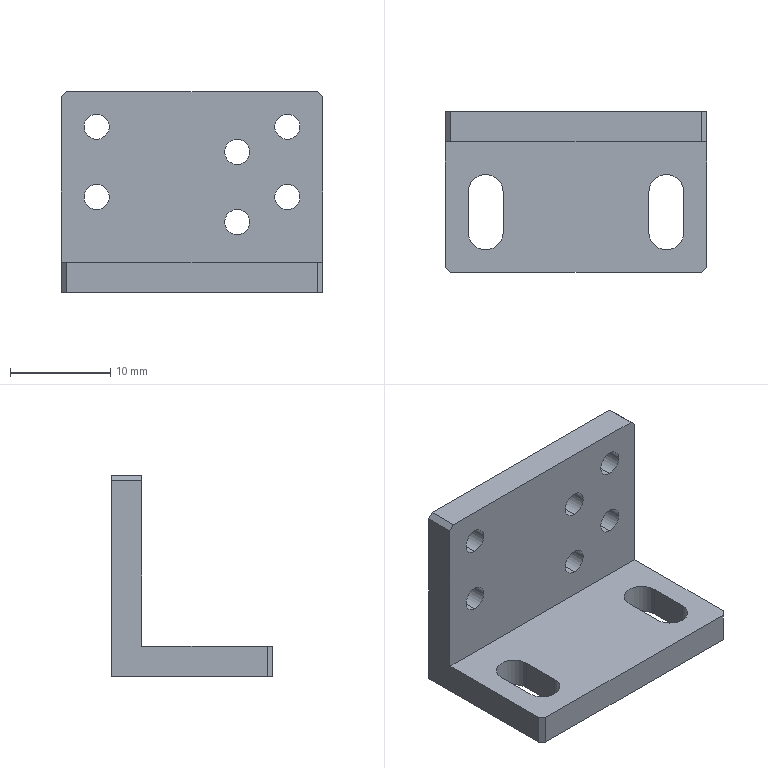Part | NX | features BREP 1 | 1 solid | 32 faces | box 26 x 16 x 20 mm | volume 2342 mm3 | plane 16 | cylinder 16 | commonest cylinder face diameters 2.5 x12 3.5 x4
STEP:
#1=CARTESIAN_POINT('',(-13.,8.,19.5));
#2=VERTEX_POINT('',#1);
#3=CARTESIAN_POINT('',(-12.5,8.,20.));
#4=VERTEX_POINT('',#3);
#5=CARTESIAN_POINT('',(-12.5,8.,20.));
#6=DIRECTION('',(0.7071,0.,0.7071));
#7=VECTOR('',#6,1000.);
#8=LINE('',#5,#7);
#9=EDGE_CURVE('',#2,#4,#8,.T.);
#10=ORIENTED_EDGE('',*,*,#9,.F.);
#11=CARTESIAN_POINT('',(-13.,5.,19.5));
#12=VERTEX_POINT('',#11);
#13=CARTESIAN_POINT('',(-13.,8.,19.5));
#14=DIRECTION('',(0.,1.,0.));
#15=VECTOR('',#14,1000.);
#16=LINE('',#13,#15);
#17=EDGE_CURVE('',#12,#2,#16,.T.);
#18=ORIENTED_EDGE('',*,*,#17,.F.);
#19=CARTESIAN_POINT('',(-12.5,5.,20.));
#20=VERTEX_POINT('',#19);
#21=CARTESIAN_POINT('',(-12.5,5.,20.));
#22=DIRECTION('',(-0.7071,0.,-0.7071));
#23=VECTOR('',#22,1000.);
#24=LINE('',#21,#23);
#25=EDGE_CURVE('',#20,#12,#24,.T.);
#26=ORIENTED_EDGE('',*,*,#25,.F.);
#27=CARTESIAN_POINT('',(-12.5,5.,20.));
#28=DIRECTION('',(0.,-1.,0.));
#29=VECTOR('',#28,1000.);
#30=LINE('',#27,#29);
#31=EDGE_CURVE('',#4,#20,#30,.T.);
#32=ORIENTED_EDGE('',*,*,#31,.F.);
#33=EDGE_LOOP('',(#10,#18,#26,#32));
#34=FACE_BOUND('',#33,.T.);
#35=CARTESIAN_POINT('',(-12.5,0.,20.));
#36=DIRECTION('',(-0.7071,0.,0.7071));
#37=DIRECTION('',(0.,1.,0.));
#38=AXIS2_PLACEMENT_3D('',#35,#36,#37);
#39=PLANE('',#38);
#40=ADVANCED_FACE('',(#34),#39,.T.);
#41=CARTESIAN_POINT('',(13.,5.,19.5));
#42=VERTEX_POINT('',#41);
#43=CARTESIAN_POINT('',(12.5,5.,20.));
#44=VERTEX_POINT('',#43);
#45=CARTESIAN_POINT('',(12.5,5.,20.));
#46=DIRECTION('',(-0.7071,0.,0.7071));
#47=VECTOR('',#46,1000.);
#48=LINE('',#45,#47);
#49=EDGE_CURVE('',#42,#44,#48,.T.);
#50=ORIENTED_EDGE('',*,*,#49,.F.);
#51=CARTESIAN_POINT('',(13.,8.,19.5));
#52=VERTEX_POINT('',#51);
#53=CARTESIAN_POINT('',(13.,5.,19.5));
#54=DIRECTION('',(0.,-1.,0.));
#55=VECTOR('',#54,1000.);
#56=LINE('',#53,#55);
#57=EDGE_CURVE('',#52,#42,#56,.T.);
#58=ORIENTED_EDGE('',*,*,#57,.F.);
#59=CARTESIAN_POINT('',(12.5,8.,20.));
#60=VERTEX_POINT('',#59);
#61=CARTESIAN_POINT('',(12.5,8.,20.));
#62=DIRECTION('',(0.7071,0.,-0.7071));
#63=VECTOR('',#62,1000.);
#64=LINE('',#61,#63);
#65=EDGE_CURVE('',#60,#52,#64,.T.);
#66=ORIENTED_EDGE('',*,*,#65,.F.);
#67=CARTESIAN_POINT('',(12.5,8.,20.));
#68=DIRECTION('',(0.,1.,0.));
#69=VECTOR('',#68,1000.);
#70=LINE('',#67,#69);
#71=EDGE_CURVE('',#44,#60,#70,.T.);
#72=ORIENTED_EDGE('',*,*,#71,.F.);
#73=EDGE_LOOP('',(#50,#58,#66,#72));
#74=FACE_BOUND('',#73,.T.);
#75=CARTESIAN_POINT('',(12.5,0.,20.));
#76=DIRECTION('',(0.7071,0.,0.7071));
#77=DIRECTION('',(0.,-1.,0.));
#78=AXIS2_PLACEMENT_3D('',#75,#76,#77);
#79=PLANE('',#78);
#80=ADVANCED_FACE('',(#74),#79,.T.);
#81=CARTESIAN_POINT('',(12.5,-8.,3.));
#82=VERTEX_POINT('',#81);
#83=CARTESIAN_POINT('',(13.,-7.5,3.));
#84=VERTEX_POINT('',#83);
#85=CARTESIAN_POINT('',(10.25,-10.25,3.));
#86=DIRECTION('',(0.7071,0.7071,0.));
#87=VECTOR('',#86,1000.);
#88=LINE('',#85,#87);
#89=EDGE_CURVE('',#82,#84,#88,.T.);
#90=ORIENTED_EDGE('',*,*,#89,.F.);
#91=CARTESIAN_POINT('',(12.5,-8.,0.));
#92=VERTEX_POINT('',#91);
#93=CARTESIAN_POINT('',(12.5,-8.,3.));
#94=DIRECTION('',(0.,0.,1.));
#95=VECTOR('',#94,1000.);
#96=LINE('',#93,#95);
#97=EDGE_CURVE('',#92,#82,#96,.T.);
#98=ORIENTED_EDGE('',*,*,#97,.F.);
#99=CARTESIAN_POINT('',(13.,-7.5,0.));
#100=VERTEX_POINT('',#99);
#101=CARTESIAN_POINT('',(13.,-7.5,0.));
#102=DIRECTION('',(-0.7071,-0.7071,0.));
#103=VECTOR('',#102,1000.);
#104=LINE('',#101,#103);
#105=EDGE_CURVE('',#100,#92,#104,.T.);
#106=ORIENTED_EDGE('',*,*,#105,.F.);
#107=CARTESIAN_POINT('',(13.,-7.5,3.));
#108=DIRECTION('',(0.,0.,-1.));
#109=VECTOR('',#108,1000.);
#110=LINE('',#107,#109);
#111=EDGE_CURVE('',#84,#100,#110,.T.);
#112=ORIENTED_EDGE('',*,*,#111,.F.);
#113=EDGE_LOOP('',(#90,#98,#106,#112));
#114=FACE_BOUND('',#113,.T.);
#115=CARTESIAN_POINT('',(13.,-7.5,3.));
#116=DIRECTION('',(-0.7071,0.7071,0.));
#117=DIRECTION('',(0.,0.,-1.));
#118=AXIS2_PLACEMENT_3D('',#115,#116,#117);
#119=PLANE('',#118);
#120=ADVANCED_FACE('',(#114),#119,.F.);
#121=CARTESIAN_POINT('',(-13.,-7.5,3.));
#122=VERTEX_POINT('',#121);
#123=CARTESIAN_POINT('',(-12.5,-8.,3.));
#124=VERTEX_POINT('',#123);
#125=CARTESIAN_POINT('',(-10.25,-10.25,3.));
#126=DIRECTION('',(0.7071,-0.7071,0.));
#127=VECTOR('',#126,1000.);
#128=LINE('',#125,#127);
#129=EDGE_CURVE('',#122,#124,#128,.T.);
#130=ORIENTED_EDGE('',*,*,#129,.F.);
#131=CARTESIAN_POINT('',(-13.,-7.5,0.));
#132=VERTEX_POINT('',#131);
#133=CARTESIAN_POINT('',(-13.,-7.5,3.));
#134=DIRECTION('',(0.,0.,1.));
#135=VECTOR('',#134,1000.);
#136=LINE('',#133,#135);
#137=EDGE_CURVE('',#132,#122,#136,.T.);
#138=ORIENTED_EDGE('',*,*,#137,.F.);
#139=CARTESIAN_POINT('',(-12.5,-8.,0.));
#140=VERTEX_POINT('',#139);
#141=CARTESIAN_POINT('',(-12.5,-8.,0.));
#142=DIRECTION('',(-0.7071,0.7071,0.));
#143=VECTOR('',#142,1000.);
#144=LINE('',#141,#143);
#145=EDGE_CURVE('',#140,#132,#144,.T.);
#146=ORIENTED_EDGE('',*,*,#145,.F.);
#147=CARTESIAN_POINT('',(-12.5,-8.,3.));
#148=DIRECTION('',(0.,0.,-1.));
#149=VECTOR('',#148,1000.);
#150=LINE('',#147,#149);
#151=EDGE_CURVE('',#124,#140,#150,.T.);
#152=ORIENTED_EDGE('',*,*,#151,.F.);
#153=EDGE_LOOP('',(#130,#138,#146,#152));
#154=FACE_BOUND('',#153,.T.);
#155=CARTESIAN_POINT('',(-12.5,-8.,3.));
#156=DIRECTION('',(0.7071,0.7071,0.));
#157=DIRECTION('',(0.,0.,-1.));
#158=AXIS2_PLACEMENT_3D('',#155,#156,#157);
#159=PLANE('',#158);
#160=ADVANCED_FACE('',(#154),#159,.F.);
#161=CARTESIAN_POINT('',(4.5,8.,15.25));
#162=VERTEX_POINT('',#161);
#163=CARTESIAN_POINT('',(4.5,5.,15.25));
#164=VERTEX_POINT('',#163);
#165=CARTESIAN_POINT('',(4.5,5.,15.25));
#166=DIRECTION('',(0.,-1.,0.));
#167=VECTOR('',#166,1000.);
#168=LINE('',#165,#167);
#169=EDGE_CURVE('',#162,#164,#168,.T.);
#170=ORIENTED_EDGE('',*,*,#169,.F.);
#171=CARTESIAN_POINT('',(4.5,8.,12.75));
#172=VERTEX_POINT('',#171);
#173=CARTESIAN_POINT('',(4.5,8.,14.));
#174=DIRECTION('',(0.,-1.,0.));
#175=DIRECTION('',(0.,0.,-1.));
#176=AXIS2_PLACEMENT_3D('',#173,#174,#175);
#177=CIRCLE('',#176,1.25);
#178=EDGE_CURVE('',#172,#162,#177,.T.);
#179=ORIENTED_EDGE('',*,*,#178,.F.);
#180=CARTESIAN_POINT('',(4.5,5.,12.75));
#181=VERTEX_POINT('',#180);
#182=CARTESIAN_POINT('',(4.5,5.,12.75));
#183=DIRECTION('',(0.,-1.,0.));
#184=VECTOR('',#183,1000.);
#185=LINE('',#182,#184);
#186=EDGE_CURVE('',#172,#181,#185,.T.);
#187=ORIENTED_EDGE('',*,*,#186,.T.);
#188=CARTESIAN_POINT('',(4.5,5.,14.));
#189=DIRECTION('',(0.,-1.,0.));
#190=DIRECTION('',(0.,0.,-1.));
#191=AXIS2_PLACEMENT_3D('',#188,#189,#190);
#192=CIRCLE('',#191,1.25);
#193=EDGE_CURVE('',#181,#164,#192,.T.);
#194=ORIENTED_EDGE('',*,*,#193,.T.);
#195=EDGE_LOOP('',(#170,#179,#187,#194));
#196=FACE_BOUND('',#195,.T.);
#197=CARTESIAN_POINT('',(4.5,5.,14.));
#198=DIRECTION('',(0.,-1.,0.));
#199=DIRECTION('',(0.,0.,-1.));
#200=AXIS2_PLACEMENT_3D('',#197,#198,#199);
#201=CYLINDRICAL_SURFACE('',#200,1.25);
#202=ADVANCED_FACE('',(#196),#201,.F.);
#203=CARTESIAN_POINT('',(4.5,8.,8.25));
#204=VERTEX_POINT('',#203);
#205=CARTESIAN_POINT('',(4.5,5.,8.25));
#206=VERTEX_POINT('',#205);
#207=CARTESIAN_POINT('',(4.5,5.,8.25));
#208=DIRECTION('',(0.,-1.,0.));
#209=VECTOR('',#208,1000.);
#210=LINE('',#207,#209);
#211=EDGE_CURVE('',#204,#206,#210,.T.);
#212=ORIENTED_EDGE('',*,*,#211,.F.);
#213=CARTESIAN_POINT('',(4.5,8.,5.75));
#214=VERTEX_POINT('',#213);
#215=CARTESIAN_POINT('',(4.5,8.,7.));
#216=DIRECTION('',(0.,-1.,0.));
#217=DIRECTION('',(0.,0.,-1.));
#218=AXIS2_PLACEMENT_3D('',#215,#216,#217);
#219=CIRCLE('',#218,1.25);
#220=EDGE_CURVE('',#214,#204,#219,.T.);
#221=ORIENTED_EDGE('',*,*,#220,.F.);
#222=CARTESIAN_POINT('',(4.5,5.,5.75));
#223=VERTEX_POINT('',#222);
#224=CARTESIAN_POINT('',(4.5,5.,5.75));
#225=DIRECTION('',(0.,-1.,0.));
#226=VECTOR('',#225,1000.);
#227=LINE('',#224,#226);
#228=EDGE_CURVE('',#214,#223,#227,.T.);
#229=ORIENTED_EDGE('',*,*,#228,.T.);
#230=CARTESIAN_POINT('',(4.5,5.,7.));
#231=DIRECTION('',(0.,-1.,0.));
#232=DIRECTION('',(0.,0.,-1.));
#233=AXIS2_PLACEMENT_3D('',#230,#231,#232);
#234=CIRCLE('',#233,1.25);
#235=EDGE_CURVE('',#223,#206,#234,.T.);
#236=ORIENTED_EDGE('',*,*,#235,.T.);
#237=EDGE_LOOP('',(#212,#221,#229,#236));
#238=FACE_BOUND('',#237,.T.);
#239=CARTESIAN_POINT('',(4.5,5.,7.));
#240=DIRECTION('',(0.,-1.,0.));
#241=DIRECTION('',(0.,0.,-1.));
#242=AXIS2_PLACEMENT_3D('',#239,#240,#241);
#243=CYLINDRICAL_SURFACE('',#242,1.25);
#244=ADVANCED_FACE('',(#238),#243,.F.);
#245=CARTESIAN_POINT('',(-9.5,8.,17.75));
#246=VERTEX_POINT('',#245);
#247=CARTESIAN_POINT('',(-9.5,5.,17.75));
#248=VERTEX_POINT('',#247);
#249=CARTESIAN_POINT('',(-9.5,5.,17.75));
#250=DIRECTION('',(0.,-1.,0.));
#251=VECTOR('',#250,1000.);
#252=LINE('',#249,#251);
#253=EDGE_CURVE('',#246,#248,#252,.T.);
#254=ORIENTED_EDGE('',*,*,#253,.F.);
#255=CARTESIAN_POINT('',(-9.5,8.,15.25));
#256=VERTEX_POINT('',#255);
#257=CARTESIAN_POINT('',(-9.5,8.,16.5));
#258=DIRECTION('',(0.,-1.,0.));
#259=DIRECTION('',(0.,0.,-1.));
#260=AXIS2_PLACEMENT_3D('',#257,#258,#259);
#261=CIRCLE('',#260,1.25);
#262=EDGE_CURVE('',#256,#246,#261,.T.);
#263=ORIENTED_EDGE('',*,*,#262,.F.);
#264=CARTESIAN_POINT('',(-9.5,5.,15.25));
#265=VERTEX_POINT('',#264);
#266=CARTESIAN_POINT('',(-9.5,5.,15.25));
#267=DIRECTION('',(0.,-1.,0.));
#268=VECTOR('',#267,1000.);
#269=LINE('',#266,#268);
#270=EDGE_CURVE('',#256,#265,#269,.T.);
#271=ORIENTED_EDGE('',*,*,#270,.T.);
#272=CARTESIAN_POINT('',(-9.5,5.,16.5));
#273=DIRECTION('',(0.,-1.,0.));
#274=DIRECTION('',(0.,0.,-1.));
#275=AXIS2_PLACEMENT_3D('',#272,#273,#274);
#276=CIRCLE('',#275,1.25);
#277=EDGE_CURVE('',#265,#248,#276,.T.);
#278=ORIENTED_EDGE('',*,*,#277,.T.);
#279=EDGE_LOOP('',(#254,#263,#271,#278));
#280=FACE_BOUND('',#279,.T.);
#281=CARTESIAN_POINT('',(-9.5,5.,16.5));
#282=DIRECTION('',(0.,-1.,0.));
#283=DIRECTION('',(0.,0.,-1.));
#284=AXIS2_PLACEMENT_3D('',#281,#282,#283);
#285=CYLINDRICAL_SURFACE('',#284,1.25);
#286=ADVANCED_FACE('',(#280),#285,.F.);
#287=CARTESIAN_POINT('',(-9.5,8.,10.75));
#288=VERTEX_POINT('',#287);
#289=CARTESIAN_POINT('',(-9.5,5.,10.75));
#290=VERTEX_POINT('',#289);
#291=CARTESIAN_POINT('',(-9.5,5.,10.75));
#292=DIRECTION('',(0.,-1.,0.));
#293=VECTOR('',#292,1000.);
#294=LINE('',#291,#293);
#295=EDGE_CURVE('',#288,#290,#294,.T.);
#296=ORIENTED_EDGE('',*,*,#295,.F.);
#297=CARTESIAN_POINT('',(-9.5,8.,8.25));
#298=VERTEX_POINT('',#297);
#299=CARTESIAN_POINT('',(-9.5,8.,9.5));
#300=DIRECTION('',(0.,-1.,0.));
#301=DIRECTION('',(0.,0.,-1.));
#302=AXIS2_PLACEMENT_3D('',#299,#300,#301);
#303=CIRCLE('',#302,1.25);
#304=EDGE_CURVE('',#298,#288,#303,.T.);
#305=ORIENTED_EDGE('',*,*,#304,.F.);
#306=CARTESIAN_POINT('',(-9.5,5.,8.25));
#307=VERTEX_POINT('',#306);
#308=CARTESIAN_POINT('',(-9.5,5.,8.25));
#309=DIRECTION('',(0.,-1.,0.));
#310=VECTOR('',#309,1000.);
#311=LINE('',#308,#310);
#312=EDGE_CURVE('',#298,#307,#311,.T.);
#313=ORIENTED_EDGE('',*,*,#312,.T.);
#314=CARTESIAN_POINT('',(-9.5,5.,9.5));
#315=DIRECTION('',(0.,-1.,0.));
#316=DIRECTION('',(0.,0.,-1.));
#317=AXIS2_PLACEMENT_3D('',#314,#315,#316);
#318=CIRCLE('',#317,1.25);
#319=EDGE_CURVE('',#307,#290,#318,.T.);
#320=ORIENTED_EDGE('',*,*,#319,.T.);
#321=EDGE_LOOP('',(#296,#305,#313,#320));
#322=FACE_BOUND('',#321,.T.);
#323=CARTESIAN_POINT('',(-9.5,5.,9.5));
#324=DIRECTION('',(0.,-1.,0.));
#325=DIRECTION('',(0.,0.,-1.));
#326=AXIS2_PLACEMENT_3D('',#323,#324,#325);
#327=CYLINDRICAL_SURFACE('',#326,1.25);
#328=ADVANCED_FACE('',(#322),#327,.F.);
#329=CARTESIAN_POINT('',(9.5,8.,17.75));
#330=VERTEX_POINT('',#329);
#331=CARTESIAN_POINT('',(9.5,5.,17.75));
#332=VERTEX_POINT('',#331);
#333=CARTESIAN_POINT('',(9.5,5.,17.75));
#334=DIRECTION('',(0.,-1.,0.));
#335=VECTOR('',#334,1000.);
#336=LINE('',#333,#335);
#337=EDGE_CURVE('',#330,#332,#336,.T.);
#338=ORIENTED_EDGE('',*,*,#337,.F.);
#339=CARTESIAN_POINT('',(9.5,8.,15.25));
#340=VERTEX_POINT('',#339);
#341=CARTESIAN_POINT('',(9.5,8.,16.5));
#342=DIRECTION('',(0.,-1.,0.));
#343=DIRECTION('',(0.,0.,-1.));
#344=AXIS2_PLACEMENT_3D('',#341,#342,#343);
#345=CIRCLE('',#344,1.25);
#346=EDGE_CURVE('',#340,#330,#345,.T.);
#347=ORIENTED_EDGE('',*,*,#346,.F.);
#348=CARTESIAN_POINT('',(9.5,5.,15.25));
#349=VERTEX_POINT('',#348);
#350=CARTESIAN_POINT('',(9.5,5.,15.25));
#351=DIRECTION('',(0.,-1.,0.));
#352=VECTOR('',#351,1000.);
#353=LINE('',#350,#352);
#354=EDGE_CURVE('',#340,#349,#353,.T.);
#355=ORIENTED_EDGE('',*,*,#354,.T.);
#356=CARTESIAN_POINT('',(9.5,5.,16.5));
#357=DIRECTION('',(0.,-1.,0.));
#358=DIRECTION('',(0.,0.,-1.));
#359=AXIS2_PLACEMENT_3D('',#356,#357,#358);
#360=CIRCLE('',#359,1.25);
#361=EDGE_CURVE('',#349,#332,#360,.T.);
#362=ORIENTED_EDGE('',*,*,#361,.T.);
#363=EDGE_LOOP('',(#338,#347,#355,#362));
#364=FACE_BOUND('',#363,.T.);
#365=CARTESIAN_POINT('',(9.5,5.,16.5));
#366=DIRECTION('',(0.,-1.,0.));
#367=DIRECTION('',(0.,0.,-1.));
#368=AXIS2_PLACEMENT_3D('',#365,#366,#367);
#369=CYLINDRICAL_SURFACE('',#368,1.25);
#370=ADVANCED_FACE('',(#364),#369,.F.);
#371=CARTESIAN_POINT('',(9.5,8.,10.75));
#372=VERTEX_POINT('',#371);
#373=CARTESIAN_POINT('',(9.5,5.,10.75));
#374=VERTEX_POINT('',#373);
#375=CARTESIAN_POINT('',(9.5,5.,10.75));
#376=DIRECTION('',(0.,-1.,0.));
#377=VECTOR('',#376,1000.);
#378=LINE('',#375,#377);
#379=EDGE_CURVE('',#372,#374,#378,.T.);
#380=ORIENTED_EDGE('',*,*,#379,.F.);
#381=CARTESIAN_POINT('',(9.5,8.,8.25));
#382=VERTEX_POINT('',#381);
#383=CARTESIAN_POINT('',(9.5,8.,9.5));
#384=DIRECTION('',(0.,-1.,0.));
#385=DIRECTION('',(0.,0.,-1.));
#386=AXIS2_PLACEMENT_3D('',#383,#384,#385);
#387=CIRCLE('',#386,1.25);
#388=EDGE_CURVE('',#382,#372,#387,.T.);
#389=ORIENTED_EDGE('',*,*,#388,.F.);
#390=CARTESIAN_POINT('',(9.5,5.,8.25));
#391=VERTEX_POINT('',#390);
#392=CARTESIAN_POINT('',(9.5,5.,8.25));
#393=DIRECTION('',(0.,-1.,0.));
#394=VECTOR('',#393,1000.);
#395=LINE('',#392,#394);
#396=EDGE_CURVE('',#382,#391,#395,.T.);
#397=ORIENTED_EDGE('',*,*,#396,.T.);
#398=CARTESIAN_POINT('',(9.5,5.,9.5));
#399=DIRECTION('',(0.,-1.,0.));
#400=DIRECTION('',(0.,0.,-1.));
#401=AXIS2_PLACEMENT_3D('',#398,#399,#400);
#402=CIRCLE('',#401,1.25);
#403=EDGE_CURVE('',#391,#374,#402,.T.);
#404=ORIENTED_EDGE('',*,*,#403,.T.);
#405=EDGE_LOOP('',(#380,#389,#397,#404));
#406=FACE_BOUND('',#405,.T.);
#407=CARTESIAN_POINT('',(9.5,5.,9.5));
#408=DIRECTION('',(0.,-1.,0.));
#409=DIRECTION('',(0.,0.,-1.));
#410=AXIS2_PLACEMENT_3D('',#407,#408,#409);
#411=CYLINDRICAL_SURFACE('',#410,1.25);
#412=ADVANCED_FACE('',(#406),#411,.F.);
#413=CARTESIAN_POINT('',(7.25,-4.,0.));
#414=VERTEX_POINT('',#413);
#415=CARTESIAN_POINT('',(7.25,0.,0.));
#416=VERTEX_POINT('',#415);
#417=CARTESIAN_POINT('',(7.25,0.,0.));
#418=DIRECTION('',(0.,1.,0.));
#419=VECTOR('',#418,1000.);
#420=LINE('',#417,#419);
#421=EDGE_CURVE('',#414,#416,#420,.T.);
#422=ORIENTED_EDGE('',*,*,#421,.T.);
#423=CARTESIAN_POINT('',(7.25,0.,3.));
#424=VERTEX_POINT('',#423);
#425=CARTESIAN_POINT('',(7.25,0.,-0.001));
#426=DIRECTION('',(0.,0.,1.));
#427=VECTOR('',#426,1000.);
#428=LINE('',#425,#427);
#429=EDGE_CURVE('',#416,#424,#428,.T.);
#430=ORIENTED_EDGE('',*,*,#429,.T.);
#431=CARTESIAN_POINT('',(7.25,-4.,3.));
#432=VERTEX_POINT('',#431);
#433=CARTESIAN_POINT('',(7.25,0.,3.));
#434=DIRECTION('',(0.,-1.,0.));
#435=VECTOR('',#434,1000.);
#436=LINE('',#433,#435);
#437=EDGE_CURVE('',#424,#432,#436,.T.);
#438=ORIENTED_EDGE('',*,*,#437,.T.);
#439=CARTESIAN_POINT('',(7.25,-4.,-0.001));
#440=DIRECTION('',(0.,0.,1.));
#441=VECTOR('',#440,1000.);
#442=LINE('',#439,#441);
#443=EDGE_CURVE('',#414,#432,#442,.T.);
#444=ORIENTED_EDGE('',*,*,#443,.F.);
#445=EDGE_LOOP('',(#422,#430,#438,#444));
#446=FACE_BOUND('',#445,.T.);
#447=CARTESIAN_POINT('',(7.25,0.,-0.001));
#448=DIRECTION('',(-1.,0.,0.));
#449=DIRECTION('',(0.,0.,1.));
#450=AXIS2_PLACEMENT_3D('',#447,#448,#449);
#451=PLANE('',#450);
#452=ADVANCED_FACE('',(#446),#451,.F.);
#453=CARTESIAN_POINT('',(10.75,-4.,0.));
#454=VERTEX_POINT('',#453);
#455=CARTESIAN_POINT('',(9.,-4.,0.));
#456=DIRECTION('',(0.,0.,-1.));
#457=DIRECTION('',(1.,0.,0.));
#458=AXIS2_PLACEMENT_3D('',#455,#456,#457);
#459=CIRCLE('',#458,1.75);
#460=EDGE_CURVE('',#454,#414,#459,.T.);
#461=ORIENTED_EDGE('',*,*,#460,.T.);
#462=ORIENTED_EDGE('',*,*,#443,.T.);
#463=CARTESIAN_POINT('',(10.75,-4.,3.));
#464=VERTEX_POINT('',#463);
#465=CARTESIAN_POINT('',(9.,-4.,3.));
#466=DIRECTION('',(0.,0.,1.));
#467=DIRECTION('',(1.,0.,0.));
#468=AXIS2_PLACEMENT_3D('',#465,#466,#467);
#469=CIRCLE('',#468,1.75);
#470=EDGE_CURVE('',#432,#464,#469,.T.);
#471=ORIENTED_EDGE('',*,*,#470,.T.);
#472=CARTESIAN_POINT('',(10.75,-4.,-0.001));
#473=DIRECTION('',(0.,0.,1.));
#474=VECTOR('',#473,1000.);
#475=LINE('',#472,#474);
#476=EDGE_CURVE('',#454,#464,#475,.T.);
#477=ORIENTED_EDGE('',*,*,#476,.F.);
#478=EDGE_LOOP('',(#461,#462,#471,#477));
#479=FACE_BOUND('',#478,.T.);
#480=CARTESIAN_POINT('',(9.,-4.,-0.001));
#481=DIRECTION('',(0.,0.,1.));
#482=DIRECTION('',(1.,0.,0.));
#483=AXIS2_PLACEMENT_3D('',#480,#481,#482);
#484=CYLINDRICAL_SURFACE('',#483,1.75);
#485=ADVANCED_FACE('',(#479),#484,.F.);
#486=CARTESIAN_POINT('',(10.75,0.,0.));
#487=VERTEX_POINT('',#486);
#488=CARTESIAN_POINT('',(10.75,0.,0.));
#489=DIRECTION('',(0.,-1.,0.));
#490=VECTOR('',#489,1000.);
#491=LINE('',#488,#490);
#492=EDGE_CURVE('',#487,#454,#491,.T.);
#493=ORIENTED_EDGE('',*,*,#492,.T.);
#494=ORIENTED_EDGE('',*,*,#476,.T.);
#495=CARTESIAN_POINT('',(10.75,0.,3.));
#496=VERTEX_POINT('',#495);
#497=CARTESIAN_POINT('',(10.75,0.,3.));
#498=DIRECTION('',(0.,1.,0.));
#499=VECTOR('',#498,1000.);
#500=LINE('',#497,#499);
#501=EDGE_CURVE('',#464,#496,#500,.T.);
#502=ORIENTED_EDGE('',*,*,#501,.T.);
#503=CARTESIAN_POINT('',(10.75,0.,-0.001));
#504=DIRECTION('',(0.,0.,1.));
#505=VECTOR('',#504,1000.);
#506=LINE('',#503,#505);
#507=EDGE_CURVE('',#487,#496,#506,.T.);
#508=ORIENTED_EDGE('',*,*,#507,.F.);
#509=EDGE_LOOP('',(#493,#494,#502,#508));
#510=FACE_BOUND('',#509,.T.);
#511=CARTESIAN_POINT('',(10.75,0.,-0.001));
#512=DIRECTION('',(1.,0.,0.));
#513=DIRECTION('',(0.,0.,-1.));
#514=AXIS2_PLACEMENT_3D('',#511,#512,#513);
#515=PLANE('',#514);
#516=ADVANCED_FACE('',(#510),#515,.F.);
#517=CARTESIAN_POINT('',(9.,0.,0.));
#518=DIRECTION('',(0.,0.,-1.));
#519=DIRECTION('',(1.,0.,0.));
#520=AXIS2_PLACEMENT_3D('',#517,#518,#519);
#521=CIRCLE('',#520,1.75);
#522=EDGE_CURVE('',#416,#487,#521,.T.);
#523=ORIENTED_EDGE('',*,*,#522,.T.);
#524=ORIENTED_EDGE('',*,*,#507,.T.);
#525=CARTESIAN_POINT('',(9.,0.,3.));
#526=DIRECTION('',(0.,0.,1.));
#527=DIRECTION('',(1.,0.,0.));
#528=AXIS2_PLACEMENT_3D('',#525,#526,#527);
#529=CIRCLE('',#528,1.75);
#530=EDGE_CURVE('',#496,#424,#529,.T.);
#531=ORIENTED_EDGE('',*,*,#530,.T.);
#532=ORIENTED_EDGE('',*,*,#429,.F.);
#533=EDGE_LOOP('',(#523,#524,#531,#532));
#534=FACE_BOUND('',#533,.T.);
#535=CARTESIAN_POINT('',(9.,0.,-0.001));
#536=DIRECTION('',(0.,0.,1.));
#537=DIRECTION('',(1.,0.,0.));
#538=AXIS2_PLACEMENT_3D('',#535,#536,#537);
#539=CYLINDRICAL_SURFACE('',#538,1.75);
#540=ADVANCED_FACE('',(#534),#539,.F.);
#541=CARTESIAN_POINT('',(-10.75,-4.,0.));
#542=VERTEX_POINT('',#541);
#543=CARTESIAN_POINT('',(-10.75,0.,0.));
#544=VERTEX_POINT('',#543);
#545=CARTESIAN_POINT('',(-10.75,0.,0.));
#546=DIRECTION('',(0.,1.,0.));
#547=VECTOR('',#546,1000.);
#548=LINE('',#545,#547);
#549=EDGE_CURVE('',#542,#544,#548,.T.);
#550=ORIENTED_EDGE('',*,*,#549,.T.);
#551=CARTESIAN_POINT('',(-10.75,0.,3.));
#552=VERTEX_POINT('',#551);
#553=CARTESIAN_POINT('',(-10.75,0.,-0.001));
#554=DIRECTION('',(0.,0.,1.));
#555=VECTOR('',#554,1000.);
#556=LINE('',#553,#555);
#557=EDGE_CURVE('',#544,#552,#556,.T.);
#558=ORIENTED_EDGE('',*,*,#557,.T.);
#559=CARTESIAN_POINT('',(-10.75,-4.,3.));
#560=VERTEX_POINT('',#559);
#561=CARTESIAN_POINT('',(-10.75,0.,3.));
#562=DIRECTION('',(0.,-1.,0.));
#563=VECTOR('',#562,1000.);
#564=LINE('',#561,#563);
#565=EDGE_CURVE('',#552,#560,#564,.T.);
#566=ORIENTED_EDGE('',*,*,#565,.T.);
#567=CARTESIAN_POINT('',(-10.75,-4.,-0.001));
#568=DIRECTION('',(0.,0.,1.));
#569=VECTOR('',#568,1000.);
#570=LINE('',#567,#569);
#571=EDGE_CURVE('',#542,#560,#570,.T.);
#572=ORIENTED_EDGE('',*,*,#571,.F.);
#573=EDGE_LOOP('',(#550,#558,#566,#572));
#574=FACE_BOUND('',#573,.T.);
#575=CARTESIAN_POINT('',(-10.75,0.,-0.001));
#576=DIRECTION('',(-1.,0.,0.));
#577=DIRECTION('',(0.,0.,1.));
#578=AXIS2_PLACEMENT_3D('',#575,#576,#577);
#579=PLANE('',#578);
#580=ADVANCED_FACE('',(#574),#579,.F.);
#581=CARTESIAN_POINT('',(-7.25,-4.,0.));
#582=VERTEX_POINT('',#581);
#583=CARTESIAN_POINT('',(-9.,-4.,0.));
#584=DIRECTION('',(0.,0.,-1.));
#585=DIRECTION('',(1.,0.,0.));
#586=AXIS2_PLACEMENT_3D('',#583,#584,#585);
#587=CIRCLE('',#586,1.75);
#588=EDGE_CURVE('',#582,#542,#587,.T.);
#589=ORIENTED_EDGE('',*,*,#588,.T.);
#590=ORIENTED_EDGE('',*,*,#571,.T.);
#591=CARTESIAN_POINT('',(-7.25,-4.,3.));
#592=VERTEX_POINT('',#591);
#593=CARTESIAN_POINT('',(-9.,-4.,3.));
#594=DIRECTION('',(0.,0.,1.));
#595=DIRECTION('',(1.,0.,0.));
#596=AXIS2_PLACEMENT_3D('',#593,#594,#595);
#597=CIRCLE('',#596,1.75);
#598=EDGE_CURVE('',#560,#592,#597,.T.);
#599=ORIENTED_EDGE('',*,*,#598,.T.);
#600=CARTESIAN_POINT('',(-7.25,-4.,-0.001));
#601=DIRECTION('',(0.,0.,1.));
#602=VECTOR('',#601,1000.);
#603=LINE('',#600,#602);
#604=EDGE_CURVE('',#582,#592,#603,.T.);
#605=ORIENTED_EDGE('',*,*,#604,.F.);
#606=EDGE_LOOP('',(#589,#590,#599,#605));
#607=FACE_BOUND('',#606,.T.);
#608=CARTESIAN_POINT('',(-9.,-4.,-0.001));
#609=DIRECTION('',(0.,0.,1.));
#610=DIRECTION('',(1.,0.,0.));
#611=AXIS2_PLACEMENT_3D('',#608,#609,#610);
#612=CYLINDRICAL_SURFACE('',#611,1.75);
#613=ADVANCED_FACE('',(#607),#612,.F.);
#614=CARTESIAN_POINT('',(-7.25,0.,0.));
#615=VERTEX_POINT('',#614);
#616=CARTESIAN_POINT('',(-7.25,0.,0.));
#617=DIRECTION('',(0.,-1.,0.));
#618=VECTOR('',#617,1000.);
#619=LINE('',#616,#618);
#620=EDGE_CURVE('',#615,#582,#619,.T.);
#621=ORIENTED_EDGE('',*,*,#620,.T.);
#622=ORIENTED_EDGE('',*,*,#604,.T.);
#623=CARTESIAN_POINT('',(-7.25,0.,3.));
#624=VERTEX_POINT('',#623);
#625=CARTESIAN_POINT('',(-7.25,0.,3.));
#626=DIRECTION('',(0.,1.,0.));
#627=VECTOR('',#626,1000.);
#628=LINE('',#625,#627);
#629=EDGE_CURVE('',#592,#624,#628,.T.);
#630=ORIENTED_EDGE('',*,*,#629,.T.);
#631=CARTESIAN_POINT('',(-7.25,0.,-0.001));
#632=DIRECTION('',(0.,0.,1.));
#633=VECTOR('',#632,1000.);
#634=LINE('',#631,#633);
#635=EDGE_CURVE('',#615,#624,#634,.T.);
#636=ORIENTED_EDGE('',*,*,#635,.F.);
#637=EDGE_LOOP('',(#621,#622,#630,#636));
#638=FACE_BOUND('',#637,.T.);
#639=CARTESIAN_POINT('',(-7.25,0.,-0.001));
#640=DIRECTION('',(1.,0.,0.));
#641=DIRECTION('',(0.,0.,-1.));
#642=AXIS2_PLACEMENT_3D('',#639,#640,#641);
#643=PLANE('',#642);
#644=ADVANCED_FACE('',(#638),#643,.F.);
#645=CARTESIAN_POINT('',(-9.,0.,0.));
#646=DIRECTION('',(0.,0.,-1.));
#647=DIRECTION('',(1.,0.,0.));
#648=AXIS2_PLACEMENT_3D('',#645,#646,#647);
#649=CIRCLE('',#648,1.75);
#650=EDGE_CURVE('',#544,#615,#649,.T.);
#651=ORIENTED_EDGE('',*,*,#650,.T.);
#652=ORIENTED_EDGE('',*,*,#635,.T.);
#653=CARTESIAN_POINT('',(-9.,0.,3.));
#654=DIRECTION('',(0.,0.,1.));
#655=DIRECTION('',(1.,0.,0.));
#656=AXIS2_PLACEMENT_3D('',#653,#654,#655);
#657=CIRCLE('',#656,1.75);
#658=EDGE_CURVE('',#624,#552,#657,.T.);
#659=ORIENTED_EDGE('',*,*,#658,.T.);
#660=ORIENTED_EDGE('',*,*,#557,.F.);
#661=EDGE_LOOP('',(#651,#652,#659,#660));
#662=FACE_BOUND('',#661,.T.);
#663=CARTESIAN_POINT('',(-9.,0.,-0.001));
#664=DIRECTION('',(0.,0.,1.));
#665=DIRECTION('',(1.,0.,0.));
#666=AXIS2_PLACEMENT_3D('',#663,#664,#665);
#667=CYLINDRICAL_SURFACE('',#666,1.75);
#668=ADVANCED_FACE('',(#662),#667,.F.);
#669=CARTESIAN_POINT('',(13.,5.,20.));
#670=DIRECTION('',(1.,0.,0.));
#671=VECTOR('',#670,1000.);
#672=LINE('',#669,#671);
#673=EDGE_CURVE('',#20,#44,#672,.T.);
#674=ORIENTED_EDGE('',*,*,#673,.T.);
#675=ORIENTED_EDGE('',*,*,#71,.T.);
#676=CARTESIAN_POINT('',(13.,8.,20.));
#677=DIRECTION('',(-1.,0.,0.));
#678=VECTOR('',#677,1000.);
#679=LINE('',#676,#678);
#680=EDGE_CURVE('',#60,#4,#679,.T.);
#681=ORIENTED_EDGE('',*,*,#680,.T.);
#682=ORIENTED_EDGE('',*,*,#31,.T.);
#683=EDGE_LOOP('',(#674,#675,#681,#682));
#684=FACE_BOUND('',#683,.T.);
#685=CARTESIAN_POINT('',(0.,0.,20.));
#686=DIRECTION('',(0.,0.,1.));
#687=DIRECTION('',(1.,0.,0.));
#688=AXIS2_PLACEMENT_3D('',#685,#686,#687);
#689=PLANE('',#688);
#690=ADVANCED_FACE('',(#684),#689,.T.);
#691=CARTESIAN_POINT('',(13.,5.,3.));
#692=VERTEX_POINT('',#691);
#693=CARTESIAN_POINT('',(13.,5.,20.));
#694=DIRECTION('',(0.,0.,-1.));
#695=VECTOR('',#694,1000.);
#696=LINE('',#693,#695);
#697=EDGE_CURVE('',#42,#692,#696,.T.);
#698=ORIENTED_EDGE('',*,*,#697,.F.);
#699=ORIENTED_EDGE('',*,*,#49,.T.);
#700=ORIENTED_EDGE('',*,*,#673,.F.);
#701=ORIENTED_EDGE('',*,*,#25,.T.);
#702=CARTESIAN_POINT('',(-13.,5.,3.));
#703=VERTEX_POINT('',#702);
#704=CARTESIAN_POINT('',(-13.,5.,20.));
#705=DIRECTION('',(0.,0.,-1.));
#706=VECTOR('',#705,1000.);
#707=LINE('',#704,#706);
#708=EDGE_CURVE('',#12,#703,#707,.T.);
#709=ORIENTED_EDGE('',*,*,#708,.T.);
#710=CARTESIAN_POINT('',(13.,5.,3.));
#711=DIRECTION('',(1.,0.,0.));
#712=VECTOR('',#711,1000.);
#713=LINE('',#710,#712);
#714=EDGE_CURVE('',#703,#692,#713,.T.);
#715=ORIENTED_EDGE('',*,*,#714,.T.);
#716=EDGE_LOOP('',(#698,#699,#700,#701,#709,#715));
#717=FACE_BOUND('',#716,.T.);
#718=ORIENTED_EDGE('',*,*,#403,.F.);
#719=CARTESIAN_POINT('',(9.5,5.,9.5));
#720=DIRECTION('',(0.,-1.,0.));
#721=DIRECTION('',(0.,0.,-1.));
#722=AXIS2_PLACEMENT_3D('',#719,#720,#721);
#723=CIRCLE('',#722,1.25);
#724=EDGE_CURVE('',#374,#391,#723,.T.);
#725=ORIENTED_EDGE('',*,*,#724,.F.);
#726=EDGE_LOOP('',(#718,#725));
#727=FACE_BOUND('',#726,.T.);
#728=ORIENTED_EDGE('',*,*,#361,.F.);
#729=CARTESIAN_POINT('',(9.5,5.,16.5));
#730=DIRECTION('',(0.,-1.,0.));
#731=DIRECTION('',(0.,0.,-1.));
#732=AXIS2_PLACEMENT_3D('',#729,#730,#731);
#733=CIRCLE('',#732,1.25);
#734=EDGE_CURVE('',#332,#349,#733,.T.);
#735=ORIENTED_EDGE('',*,*,#734,.F.);
#736=EDGE_LOOP('',(#728,#735));
#737=FACE_BOUND('',#736,.T.);
#738=ORIENTED_EDGE('',*,*,#319,.F.);
#739=CARTESIAN_POINT('',(-9.5,5.,9.5));
#740=DIRECTION('',(0.,-1.,0.));
#741=DIRECTION('',(0.,0.,-1.));
#742=AXIS2_PLACEMENT_3D('',#739,#740,#741);
#743=CIRCLE('',#742,1.25);
#744=EDGE_CURVE('',#290,#307,#743,.T.);
#745=ORIENTED_EDGE('',*,*,#744,.F.);
#746=EDGE_LOOP('',(#738,#745));
#747=FACE_BOUND('',#746,.T.);
#748=ORIENTED_EDGE('',*,*,#277,.F.);
#749=CARTESIAN_POINT('',(-9.5,5.,16.5));
#750=DIRECTION('',(0.,-1.,0.));
#751=DIRECTION('',(0.,0.,-1.));
#752=AXIS2_PLACEMENT_3D('',#749,#750,#751);
#753=CIRCLE('',#752,1.25);
#754=EDGE_CURVE('',#248,#265,#753,.T.);
#755=ORIENTED_EDGE('',*,*,#754,.F.);
#756=EDGE_LOOP('',(#748,#755));
#757=FACE_BOUND('',#756,.T.);
#758=ORIENTED_EDGE('',*,*,#235,.F.);
#759=CARTESIAN_POINT('',(4.5,5.,7.));
#760=DIRECTION('',(0.,-1.,0.));
#761=DIRECTION('',(0.,0.,-1.));
#762=AXIS2_PLACEMENT_3D('',#759,#760,#761);
#763=CIRCLE('',#762,1.25);
#764=EDGE_CURVE('',#206,#223,#763,.T.);
#765=ORIENTED_EDGE('',*,*,#764,.F.);
#766=EDGE_LOOP('',(#758,#765));
#767=FACE_BOUND('',#766,.T.);
#768=ORIENTED_EDGE('',*,*,#193,.F.);
#769=CARTESIAN_POINT('',(4.5,5.,14.));
#770=DIRECTION('',(0.,-1.,0.));
#771=DIRECTION('',(0.,0.,-1.));
#772=AXIS2_PLACEMENT_3D('',#769,#770,#771);
#773=CIRCLE('',#772,1.25);
#774=EDGE_CURVE('',#164,#181,#773,.T.);
#775=ORIENTED_EDGE('',*,*,#774,.F.);
#776=EDGE_LOOP('',(#768,#775));
#777=FACE_BOUND('',#776,.T.);
#778=CARTESIAN_POINT('',(13.,5.,20.));
#779=DIRECTION('',(0.,1.,0.));
#780=DIRECTION('',(0.,0.,1.));
#781=AXIS2_PLACEMENT_3D('',#778,#779,#780);
#782=PLANE('',#781);
#783=ADVANCED_FACE('',(#717,#727,#737,#747,#757,#767,#777),#782,.F.);
#784=CARTESIAN_POINT('',(-13.,-8.,0.));
#785=DIRECTION('',(1.,0.,0.));
#786=VECTOR('',#785,1000.);
#787=LINE('',#784,#786);
#788=EDGE_CURVE('',#140,#92,#787,.T.);
#789=ORIENTED_EDGE('',*,*,#788,.F.);
#790=ORIENTED_EDGE('',*,*,#145,.T.);
#791=CARTESIAN_POINT('',(-13.,8.,0.));
#792=VERTEX_POINT('',#791);
#793=CARTESIAN_POINT('',(-13.,8.,0.));
#794=DIRECTION('',(0.,-1.,0.));
#795=VECTOR('',#794,1000.);
#796=LINE('',#793,#795);
#797=EDGE_CURVE('',#792,#132,#796,.T.);
#798=ORIENTED_EDGE('',*,*,#797,.F.);
#799=CARTESIAN_POINT('',(13.,8.,0.));
#800=VERTEX_POINT('',#799);
#801=CARTESIAN_POINT('',(-13.,8.,0.));
#802=DIRECTION('',(-1.,0.,0.));
#803=VECTOR('',#802,1000.);
#804=LINE('',#801,#803);
#805=EDGE_CURVE('',#800,#792,#804,.T.);
#806=ORIENTED_EDGE('',*,*,#805,.F.);
#807=CARTESIAN_POINT('',(13.,8.,0.));
#808=DIRECTION('',(0.,1.,0.));
#809=VECTOR('',#808,1000.);
#810=LINE('',#807,#809);
#811=EDGE_CURVE('',#100,#800,#810,.T.);
#812=ORIENTED_EDGE('',*,*,#811,.F.);
#813=ORIENTED_EDGE('',*,*,#105,.T.);
#814=EDGE_LOOP('',(#789,#790,#798,#806,#812,#813));
#815=FACE_BOUND('',#814,.T.);
#816=ORIENTED_EDGE('',*,*,#620,.F.);
#817=ORIENTED_EDGE('',*,*,#650,.F.);
#818=ORIENTED_EDGE('',*,*,#549,.F.);
#819=ORIENTED_EDGE('',*,*,#588,.F.);
#820=EDGE_LOOP('',(#816,#817,#818,#819));
#821=FACE_BOUND('',#820,.T.);
#822=ORIENTED_EDGE('',*,*,#492,.F.);
#823=ORIENTED_EDGE('',*,*,#522,.F.);
#824=ORIENTED_EDGE('',*,*,#421,.F.);
#825=ORIENTED_EDGE('',*,*,#460,.F.);
#826=EDGE_LOOP('',(#822,#823,#824,#825));
#827=FACE_BOUND('',#826,.T.);
#828=CARTESIAN_POINT('',(0.,0.,0.));
#829=DIRECTION('',(0.,0.,1.));
#830=DIRECTION('',(1.,0.,0.));
#831=AXIS2_PLACEMENT_3D('',#828,#829,#830);
#832=PLANE('',#831);
#833=ADVANCED_FACE('',(#815,#821,#827),#832,.F.);
#834=CARTESIAN_POINT('',(-13.,8.,3.));
#835=DIRECTION('',(0.,-1.,0.));
#836=VECTOR('',#835,1000.);
#837=LINE('',#834,#836);
#838=EDGE_CURVE('',#703,#122,#837,.T.);
#839=ORIENTED_EDGE('',*,*,#838,.T.);
#840=ORIENTED_EDGE('',*,*,#129,.T.);
#841=CARTESIAN_POINT('',(-13.,-8.,3.));
#842=DIRECTION('',(1.,0.,0.));
#843=VECTOR('',#842,1000.);
#844=LINE('',#841,#843);
#845=EDGE_CURVE('',#124,#82,#844,.T.);
#846=ORIENTED_EDGE('',*,*,#845,.T.);
#847=ORIENTED_EDGE('',*,*,#89,.T.);
#848=CARTESIAN_POINT('',(13.,8.,3.));
#849=DIRECTION('',(0.,1.,0.));
#850=VECTOR('',#849,1000.);
#851=LINE('',#848,#850);
#852=EDGE_CURVE('',#84,#692,#851,.T.);
#853=ORIENTED_EDGE('',*,*,#852,.T.);
#854=ORIENTED_EDGE('',*,*,#714,.F.);
#855=EDGE_LOOP('',(#839,#840,#846,#847,#853,#854));
#856=FACE_BOUND('',#855,.T.);
#857=ORIENTED_EDGE('',*,*,#658,.F.);
#858=ORIENTED_EDGE('',*,*,#629,.F.);
#859=ORIENTED_EDGE('',*,*,#598,.F.);
#860=ORIENTED_EDGE('',*,*,#565,.F.);
#861=EDGE_LOOP('',(#857,#858,#859,#860));
#862=FACE_BOUND('',#861,.T.);
#863=ORIENTED_EDGE('',*,*,#530,.F.);
#864=ORIENTED_EDGE('',*,*,#501,.F.);
#865=ORIENTED_EDGE('',*,*,#470,.F.);
#866=ORIENTED_EDGE('',*,*,#437,.F.);
#867=EDGE_LOOP('',(#863,#864,#865,#866));
#868=FACE_BOUND('',#867,.T.);
#869=CARTESIAN_POINT('',(0.,0.,3.));
#870=DIRECTION('',(0.,0.,1.));
#871=DIRECTION('',(1.,0.,0.));
#872=AXIS2_PLACEMENT_3D('',#869,#870,#871);
#873=PLANE('',#872);
#874=ADVANCED_FACE('',(#856,#862,#868),#873,.T.);
#875=ORIENTED_EDGE('',*,*,#845,.F.);
#876=ORIENTED_EDGE('',*,*,#151,.T.);
#877=ORIENTED_EDGE('',*,*,#788,.T.);
#878=ORIENTED_EDGE('',*,*,#97,.T.);
#879=EDGE_LOOP('',(#875,#876,#877,#878));
#880=FACE_BOUND('',#879,.T.);
#881=CARTESIAN_POINT('',(-13.,-8.,3.));
#882=DIRECTION('',(0.,1.,0.));
#883=DIRECTION('',(0.,0.,1.));
#884=AXIS2_PLACEMENT_3D('',#881,#882,#883);
#885=PLANE('',#884);
#886=ADVANCED_FACE('',(#880),#885,.F.);
#887=ORIENTED_EDGE('',*,*,#797,.T.);
#888=ORIENTED_EDGE('',*,*,#137,.T.);
#889=ORIENTED_EDGE('',*,*,#838,.F.);
#890=ORIENTED_EDGE('',*,*,#708,.F.);
#891=ORIENTED_EDGE('',*,*,#17,.T.);
#892=CARTESIAN_POINT('',(-13.,8.,3.));
#893=DIRECTION('',(0.,0.,-1.));
#894=VECTOR('',#893,1000.);
#895=LINE('',#892,#894);
#896=EDGE_CURVE('',#2,#792,#895,.T.);
#897=ORIENTED_EDGE('',*,*,#896,.T.);
#898=EDGE_LOOP('',(#887,#888,#889,#890,#891,#897));
#899=FACE_BOUND('',#898,.T.);
#900=CARTESIAN_POINT('',(-13.,8.,3.));
#901=DIRECTION('',(1.,0.,0.));
#902=DIRECTION('',(0.,1.,0.));
#903=AXIS2_PLACEMENT_3D('',#900,#901,#902);
#904=PLANE('',#903);
#905=ADVANCED_FACE('',(#899),#904,.F.);
#906=ORIENTED_EDGE('',*,*,#680,.F.);
#907=ORIENTED_EDGE('',*,*,#65,.T.);
#908=CARTESIAN_POINT('',(13.,8.,3.));
#909=DIRECTION('',(0.,0.,-1.));
#910=VECTOR('',#909,1000.);
#911=LINE('',#908,#910);
#912=EDGE_CURVE('',#52,#800,#911,.T.);
#913=ORIENTED_EDGE('',*,*,#912,.T.);
#914=ORIENTED_EDGE('',*,*,#805,.T.);
#915=ORIENTED_EDGE('',*,*,#896,.F.);
#916=ORIENTED_EDGE('',*,*,#9,.T.);
#917=EDGE_LOOP('',(#906,#907,#913,#914,#915,#916));
#918=FACE_BOUND('',#917,.T.);
#919=ORIENTED_EDGE('',*,*,#388,.T.);
#920=CARTESIAN_POINT('',(9.5,8.,9.5));
#921=DIRECTION('',(0.,-1.,0.));
#922=DIRECTION('',(0.,0.,-1.));
#923=AXIS2_PLACEMENT_3D('',#920,#921,#922);
#924=CIRCLE('',#923,1.25);
#925=EDGE_CURVE('',#372,#382,#924,.T.);
#926=ORIENTED_EDGE('',*,*,#925,.T.);
#927=EDGE_LOOP('',(#919,#926));
#928=FACE_BOUND('',#927,.T.);
#929=ORIENTED_EDGE('',*,*,#346,.T.);
#930=CARTESIAN_POINT('',(9.5,8.,16.5));
#931=DIRECTION('',(0.,-1.,0.));
#932=DIRECTION('',(0.,0.,-1.));
#933=AXIS2_PLACEMENT_3D('',#930,#931,#932);
#934=CIRCLE('',#933,1.25);
#935=EDGE_CURVE('',#330,#340,#934,.T.);
#936=ORIENTED_EDGE('',*,*,#935,.T.);
#937=EDGE_LOOP('',(#929,#936));
#938=FACE_BOUND('',#937,.T.);
#939=ORIENTED_EDGE('',*,*,#304,.T.);
#940=CARTESIAN_POINT('',(-9.5,8.,9.5));
#941=DIRECTION('',(0.,-1.,0.));
#942=DIRECTION('',(0.,0.,-1.));
#943=AXIS2_PLACEMENT_3D('',#940,#941,#942);
#944=CIRCLE('',#943,1.25);
#945=EDGE_CURVE('',#288,#298,#944,.T.);
#946=ORIENTED_EDGE('',*,*,#945,.T.);
#947=EDGE_LOOP('',(#939,#946));
#948=FACE_BOUND('',#947,.T.);
#949=ORIENTED_EDGE('',*,*,#262,.T.);
#950=CARTESIAN_POINT('',(-9.5,8.,16.5));
#951=DIRECTION('',(0.,-1.,0.));
#952=DIRECTION('',(0.,0.,-1.));
#953=AXIS2_PLACEMENT_3D('',#950,#951,#952);
#954=CIRCLE('',#953,1.25);
#955=EDGE_CURVE('',#246,#256,#954,.T.);
#956=ORIENTED_EDGE('',*,*,#955,.T.);
#957=EDGE_LOOP('',(#949,#956));
#958=FACE_BOUND('',#957,.T.);
#959=ORIENTED_EDGE('',*,*,#220,.T.);
#960=CARTESIAN_POINT('',(4.5,8.,7.));
#961=DIRECTION('',(0.,-1.,0.));
#962=DIRECTION('',(0.,0.,-1.));
#963=AXIS2_PLACEMENT_3D('',#960,#961,#962);
#964=CIRCLE('',#963,1.25);
#965=EDGE_CURVE('',#204,#214,#964,.T.);
#966=ORIENTED_EDGE('',*,*,#965,.T.);
#967=EDGE_LOOP('',(#959,#966));
#968=FACE_BOUND('',#967,.T.);
#969=ORIENTED_EDGE('',*,*,#178,.T.);
#970=CARTESIAN_POINT('',(4.5,8.,14.));
#971=DIRECTION('',(0.,-1.,0.));
#972=DIRECTION('',(0.,0.,-1.));
#973=AXIS2_PLACEMENT_3D('',#970,#971,#972);
#974=CIRCLE('',#973,1.25);
#975=EDGE_CURVE('',#162,#172,#974,.T.);
#976=ORIENTED_EDGE('',*,*,#975,.T.);
#977=EDGE_LOOP('',(#969,#976));
#978=FACE_BOUND('',#977,.T.);
#979=CARTESIAN_POINT('',(-13.,8.,3.));
#980=DIRECTION('',(0.,-1.,0.));
#981=DIRECTION('',(0.,0.,-1.));
#982=AXIS2_PLACEMENT_3D('',#979,#980,#981);
#983=PLANE('',#982);
#984=ADVANCED_FACE('',(#918,#928,#938,#948,#958,#968,#978),#983,.F.);
#985=ORIENTED_EDGE('',*,*,#852,.F.);
#986=ORIENTED_EDGE('',*,*,#111,.T.);
#987=ORIENTED_EDGE('',*,*,#811,.T.);
#988=ORIENTED_EDGE('',*,*,#912,.F.);
#989=ORIENTED_EDGE('',*,*,#57,.T.);
#990=ORIENTED_EDGE('',*,*,#697,.T.);
#991=EDGE_LOOP('',(#985,#986,#987,#988,#989,#990));
#992=FACE_BOUND('',#991,.T.);
#993=CARTESIAN_POINT('',(13.,8.,3.));
#994=DIRECTION('',(-1.,0.,0.));
#995=DIRECTION('',(0.,-1.,0.));
#996=AXIS2_PLACEMENT_3D('',#993,#994,#995);
#997=PLANE('',#996);
#998=ADVANCED_FACE('',(#992),#997,.F.);
#999=ORIENTED_EDGE('',*,*,#925,.F.);
#1000=ORIENTED_EDGE('',*,*,#379,.T.);
#1001=ORIENTED_EDGE('',*,*,#724,.T.);
#1002=ORIENTED_EDGE('',*,*,#396,.F.);
#1003=EDGE_LOOP('',(#999,#1000,#1001,#1002));
#1004=FACE_BOUND('',#1003,.T.);
#1005=CARTESIAN_POINT('',(9.5,5.,9.5));
#1006=DIRECTION('',(0.,-1.,0.));
#1007=DIRECTION('',(0.,0.,-1.));
#1008=AXIS2_PLACEMENT_3D('',#1005,#1006,#1007);
#1009=CYLINDRICAL_SURFACE('',#1008,1.25);
#1010=ADVANCED_FACE('',(#1004),#1009,.F.);
#1011=ORIENTED_EDGE('',*,*,#935,.F.);
#1012=ORIENTED_EDGE('',*,*,#337,.T.);
#1013=ORIENTED_EDGE('',*,*,#734,.T.);
#1014=ORIENTED_EDGE('',*,*,#354,.F.);
#1015=EDGE_LOOP('',(#1011,#1012,#1013,#1014));
#1016=FACE_BOUND('',#1015,.T.);
#1017=CARTESIAN_POINT('',(9.5,5.,16.5));
#1018=DIRECTION('',(0.,-1.,0.));
#1019=DIRECTION('',(0.,0.,-1.));
#1020=AXIS2_PLACEMENT_3D('',#1017,#1018,#1019);
#1021=CYLINDRICAL_SURFACE('',#1020,1.25);
#1022=ADVANCED_FACE('',(#1016),#1021,.F.);
#1023=ORIENTED_EDGE('',*,*,#945,.F.);
#1024=ORIENTED_EDGE('',*,*,#295,.T.);
#1025=ORIENTED_EDGE('',*,*,#744,.T.);
#1026=ORIENTED_EDGE('',*,*,#312,.F.);
#1027=EDGE_LOOP('',(#1023,#1024,#1025,#1026));
#1028=FACE_BOUND('',#1027,.T.);
#1029=CARTESIAN_POINT('',(-9.5,5.,9.5));
#1030=DIRECTION('',(0.,-1.,0.));
#1031=DIRECTION('',(0.,0.,-1.));
#1032=AXIS2_PLACEMENT_3D('',#1029,#1030,#1031);
#1033=CYLINDRICAL_SURFACE('',#1032,1.25);
#1034=ADVANCED_FACE('',(#1028),#1033,.F.);
#1035=ORIENTED_EDGE('',*,*,#955,.F.);
#1036=ORIENTED_EDGE('',*,*,#253,.T.);
#1037=ORIENTED_EDGE('',*,*,#754,.T.);
#1038=ORIENTED_EDGE('',*,*,#270,.F.);
#1039=EDGE_LOOP('',(#1035,#1036,#1037,#1038));
#1040=FACE_BOUND('',#1039,.T.);
#1041=CARTESIAN_POINT('',(-9.5,5.,16.5));
#1042=DIRECTION('',(0.,-1.,0.));
#1043=DIRECTION('',(0.,0.,-1.));
#1044=AXIS2_PLACEMENT_3D('',#1041,#1042,#1043);
#1045=CYLINDRICAL_SURFACE('',#1044,1.25);
#1046=ADVANCED_FACE('',(#1040),#1045,.F.);
#1047=ORIENTED_EDGE('',*,*,#965,.F.);
#1048=ORIENTED_EDGE('',*,*,#211,.T.);
#1049=ORIENTED_EDGE('',*,*,#764,.T.);
#1050=ORIENTED_EDGE('',*,*,#228,.F.);
#1051=EDGE_LOOP('',(#1047,#1048,#1049,#1050));
#1052=FACE_BOUND('',#1051,.T.);
#1053=CARTESIAN_POINT('',(4.5,5.,7.));
#1054=DIRECTION('',(0.,-1.,0.));
#1055=DIRECTION('',(0.,0.,-1.));
#1056=AXIS2_PLACEMENT_3D('',#1053,#1054,#1055);
#1057=CYLINDRICAL_SURFACE('',#1056,1.25);
#1058=ADVANCED_FACE('',(#1052),#1057,.F.);
#1059=ORIENTED_EDGE('',*,*,#975,.F.);
#1060=ORIENTED_EDGE('',*,*,#169,.T.);
#1061=ORIENTED_EDGE('',*,*,#774,.T.);
#1062=ORIENTED_EDGE('',*,*,#186,.F.);
#1063=EDGE_LOOP('',(#1059,#1060,#1061,#1062));
#1064=FACE_BOUND('',#1063,.T.);
#1065=CARTESIAN_POINT('',(4.5,5.,14.));
#1066=DIRECTION('',(0.,-1.,0.));
#1067=DIRECTION('',(0.,0.,-1.));
#1068=AXIS2_PLACEMENT_3D('',#1065,#1066,#1067);
#1069=CYLINDRICAL_SURFACE('',#1068,1.25);
#1070=ADVANCED_FACE('',(#1064),#1069,.F.);
#1071=CLOSED_SHELL('',(#40,#80,#120,#160,#202,#244,#286,#328,#370,#412,#452,#485,#516,#540,#580,#613,#644,#668,#690,#783,#833,#874,#886,#905,#984,#998,#1010,#1022,#1034,#1046,#1058,#1070));
#1072=MANIFOLD_SOLID_BREP('',#1071);
#1073=(LENGTH_UNIT()NAMED_UNIT(*)SI_UNIT(.MILLI.,.METRE.));
#1074=UNCERTAINTY_MEASURE_WITH_UNIT(LENGTH_MEASURE(0.00001),#1073,'','');
#1075=(NAMED_UNIT(*)PLANE_ANGLE_UNIT()SI_UNIT($,.RADIAN.));
#1076=(NAMED_UNIT(*)SI_UNIT($,.STERADIAN.)SOLID_ANGLE_UNIT());
#1077=(GEOMETRIC_REPRESENTATION_CONTEXT(3)GLOBAL_UNCERTAINTY_ASSIGNED_CONTEXT((#1074))GLOBAL_UNIT_ASSIGNED_CONTEXT((#1073,#1075,#1076))REPRESENTATION_CONTEXT('',''));
#1078=ADVANCED_BREP_SHAPE_REPRESENTATION('',(#1072),#1077);